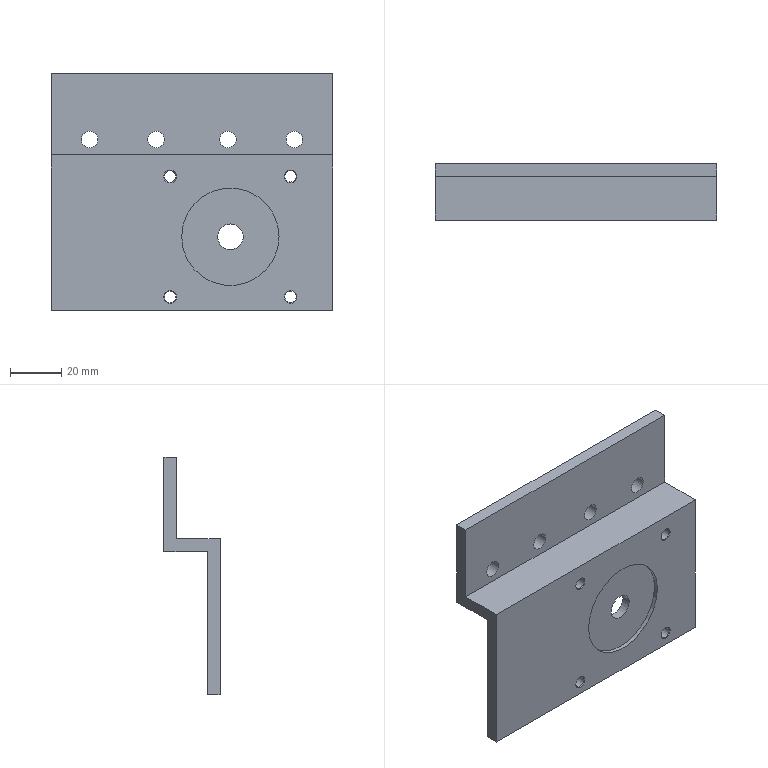Part | NX | features SIMPLE HOLE 10, DATUM_CSYS 5, SKETCH 4, SYMBOLIC_THREAD 4, HOLE PACKAGE 3, EXTRUDE 2 | 1 solid | 29 faces | box 110 x 22 x 93 mm | volume 57423 mm3 | plane 11 | cylinder 10 | cone 8 | commonest cylinder face diameters 4.5 x4 6.5 x4 10 x1 38.1 x1
STEP:
#1=CARTESIAN_POINT('',(38.55,0.,55.1));
#2=VERTEX_POINT('',#1);
#3=CARTESIAN_POINT('',(38.55,0.,52.6));
#4=DIRECTION('',(0.,1.,0.));
#5=DIRECTION('',(0.,0.,1.));
#6=AXIS2_PLACEMENT_3D('',#3,#4,#5);
#7=CIRCLE('',#6,2.5);
#8=EDGE_CURVE('',#2,#2,#7,.T.);
#9=ORIENTED_EDGE('',*,*,#8,.T.);
#10=EDGE_LOOP('',(#9));
#11=FACE_BOUND('',#10,.T.);
#12=CARTESIAN_POINT('',(38.55,0.,8.));
#13=VERTEX_POINT('',#12);
#14=CARTESIAN_POINT('',(38.55,0.,5.5));
#15=DIRECTION('',(0.,1.,0.));
#16=DIRECTION('',(0.,0.,1.));
#17=AXIS2_PLACEMENT_3D('',#14,#15,#16);
#18=CIRCLE('',#17,2.5);
#19=EDGE_CURVE('',#13,#13,#18,.T.);
#20=ORIENTED_EDGE('',*,*,#19,.T.);
#21=EDGE_LOOP('',(#20));
#22=FACE_BOUND('',#21,.T.);
#23=CARTESIAN_POINT('',(-8.55,0.,55.05));
#24=VERTEX_POINT('',#23);
#25=CARTESIAN_POINT('',(-8.55,0.,52.55));
#26=DIRECTION('',(0.,1.,0.));
#27=DIRECTION('',(0.,0.,1.));
#28=AXIS2_PLACEMENT_3D('',#25,#26,#27);
#29=CIRCLE('',#28,2.5);
#30=EDGE_CURVE('',#24,#24,#29,.T.);
#31=ORIENTED_EDGE('',*,*,#30,.T.);
#32=EDGE_LOOP('',(#31));
#33=FACE_BOUND('',#32,.T.);
#34=CARTESIAN_POINT('',(-8.55,0.,7.95));
#35=VERTEX_POINT('',#34);
#36=CARTESIAN_POINT('',(-8.55,0.,5.45));
#37=DIRECTION('',(0.,1.,0.));
#38=DIRECTION('',(0.,0.,1.));
#39=AXIS2_PLACEMENT_3D('',#36,#37,#38);
#40=CIRCLE('',#39,2.5);
#41=EDGE_CURVE('',#35,#35,#40,.T.);
#42=ORIENTED_EDGE('',*,*,#41,.T.);
#43=EDGE_LOOP('',(#42));
#44=FACE_BOUND('',#43,.T.);
#45=CARTESIAN_POINT('',(34.05,0.,29.));
#46=VERTEX_POINT('',#45);
#47=CARTESIAN_POINT('',(15.,0.,29.));
#48=DIRECTION('',(0.,-1.,0.));
#49=DIRECTION('',(1.,0.,0.));
#50=AXIS2_PLACEMENT_3D('',#47,#48,#49);
#51=CIRCLE('',#50,19.05);
#52=EDGE_CURVE('',#46,#46,#51,.T.);
#53=ORIENTED_EDGE('',*,*,#52,.F.);
#54=EDGE_LOOP('',(#53));
#55=FACE_BOUND('',#54,.T.);
#56=CARTESIAN_POINT('',(-55.,0.,61.));
#57=VERTEX_POINT('',#56);
#58=CARTESIAN_POINT('',(-55.,0.,0.));
#59=VERTEX_POINT('',#58);
#60=CARTESIAN_POINT('',(-55.,0.,61.));
#61=DIRECTION('',(0.,0.,-1.));
#62=VECTOR('',#61,1000.);
#63=LINE('',#60,#62);
#64=EDGE_CURVE('',#57,#59,#63,.T.);
#65=ORIENTED_EDGE('',*,*,#64,.T.);
#66=CARTESIAN_POINT('',(55.,0.,0.));
#67=VERTEX_POINT('',#66);
#68=CARTESIAN_POINT('',(55.,0.,0.));
#69=DIRECTION('',(-1.,0.,0.));
#70=VECTOR('',#69,1000.);
#71=LINE('',#68,#70);
#72=EDGE_CURVE('',#67,#59,#71,.T.);
#73=ORIENTED_EDGE('',*,*,#72,.F.);
#74=CARTESIAN_POINT('',(55.,0.,61.));
#75=VERTEX_POINT('',#74);
#76=CARTESIAN_POINT('',(55.,0.,61.));
#77=DIRECTION('',(0.,0.,-1.));
#78=VECTOR('',#77,1000.);
#79=LINE('',#76,#78);
#80=EDGE_CURVE('',#75,#67,#79,.T.);
#81=ORIENTED_EDGE('',*,*,#80,.F.);
#82=CARTESIAN_POINT('',(55.,0.,61.));
#83=DIRECTION('',(-1.,0.,0.));
#84=VECTOR('',#83,1000.);
#85=LINE('',#82,#84);
#86=EDGE_CURVE('',#75,#57,#85,.T.);
#87=ORIENTED_EDGE('',*,*,#86,.T.);
#88=EDGE_LOOP('',(#65,#73,#81,#87));
#89=FACE_BOUND('',#88,.T.);
#90=CARTESIAN_POINT('',(55.,0.,61.));
#91=DIRECTION('',(0.,1.,0.));
#92=DIRECTION('',(0.,0.,1.));
#93=AXIS2_PLACEMENT_3D('',#90,#91,#92);
#94=PLANE('',#93);
#95=ADVANCED_FACE('',(#11,#22,#33,#44,#55,#89),#94,.F.);
#96=CARTESIAN_POINT('',(-55.,5.,0.));
#97=VERTEX_POINT('',#96);
#98=CARTESIAN_POINT('',(-55.,0.,0.));
#99=DIRECTION('',(0.,1.,0.));
#100=VECTOR('',#99,1000.);
#101=LINE('',#98,#100);
#102=EDGE_CURVE('',#59,#97,#101,.T.);
#103=ORIENTED_EDGE('',*,*,#102,.T.);
#104=CARTESIAN_POINT('',(55.,5.,0.));
#105=VERTEX_POINT('',#104);
#106=CARTESIAN_POINT('',(55.,5.,0.));
#107=DIRECTION('',(-1.,0.,0.));
#108=VECTOR('',#107,1000.);
#109=LINE('',#106,#108);
#110=EDGE_CURVE('',#105,#97,#109,.T.);
#111=ORIENTED_EDGE('',*,*,#110,.F.);
#112=CARTESIAN_POINT('',(55.,0.,0.));
#113=DIRECTION('',(0.,1.,0.));
#114=VECTOR('',#113,1000.);
#115=LINE('',#112,#114);
#116=EDGE_CURVE('',#67,#105,#115,.T.);
#117=ORIENTED_EDGE('',*,*,#116,.F.);
#118=ORIENTED_EDGE('',*,*,#72,.T.);
#119=EDGE_LOOP('',(#103,#111,#117,#118));
#120=FACE_BOUND('',#119,.T.);
#121=CARTESIAN_POINT('',(55.,0.,0.));
#122=DIRECTION('',(0.,0.,1.));
#123=DIRECTION('',(0.,-1.,0.));
#124=AXIS2_PLACEMENT_3D('',#121,#122,#123);
#125=PLANE('',#124);
#126=ADVANCED_FACE('',(#120),#125,.F.);
#127=CARTESIAN_POINT('',(38.55,5.,50.1));
#128=VERTEX_POINT('',#127);
#129=CARTESIAN_POINT('',(38.55,5.,52.6));
#130=DIRECTION('',(0.,-1.,0.));
#131=DIRECTION('',(0.,0.,-1.));
#132=AXIS2_PLACEMENT_3D('',#129,#130,#131);
#133=CIRCLE('',#132,2.5);
#134=EDGE_CURVE('',#128,#128,#133,.T.);
#135=ORIENTED_EDGE('',*,*,#134,.T.);
#136=EDGE_LOOP('',(#135));
#137=FACE_BOUND('',#136,.T.);
#138=CARTESIAN_POINT('',(38.55,5.,3.));
#139=VERTEX_POINT('',#138);
#140=CARTESIAN_POINT('',(38.55,5.,5.5));
#141=DIRECTION('',(0.,-1.,0.));
#142=DIRECTION('',(0.,0.,-1.));
#143=AXIS2_PLACEMENT_3D('',#140,#141,#142);
#144=CIRCLE('',#143,2.5);
#145=EDGE_CURVE('',#139,#139,#144,.T.);
#146=ORIENTED_EDGE('',*,*,#145,.T.);
#147=EDGE_LOOP('',(#146));
#148=FACE_BOUND('',#147,.T.);
#149=CARTESIAN_POINT('',(-8.55,5.,50.05));
#150=VERTEX_POINT('',#149);
#151=CARTESIAN_POINT('',(-8.55,5.,52.55));
#152=DIRECTION('',(0.,-1.,0.));
#153=DIRECTION('',(0.,0.,-1.));
#154=AXIS2_PLACEMENT_3D('',#151,#152,#153);
#155=CIRCLE('',#154,2.5);
#156=EDGE_CURVE('',#150,#150,#155,.T.);
#157=ORIENTED_EDGE('',*,*,#156,.T.);
#158=EDGE_LOOP('',(#157));
#159=FACE_BOUND('',#158,.T.);
#160=CARTESIAN_POINT('',(-8.55,5.,2.95));
#161=VERTEX_POINT('',#160);
#162=CARTESIAN_POINT('',(-8.55,5.,5.45));
#163=DIRECTION('',(0.,-1.,0.));
#164=DIRECTION('',(0.,0.,-1.));
#165=AXIS2_PLACEMENT_3D('',#162,#163,#164);
#166=CIRCLE('',#165,2.5);
#167=EDGE_CURVE('',#161,#161,#166,.T.);
#168=ORIENTED_EDGE('',*,*,#167,.T.);
#169=EDGE_LOOP('',(#168));
#170=FACE_BOUND('',#169,.T.);
#171=CARTESIAN_POINT('',(15.,5.,24.));
#172=VERTEX_POINT('',#171);
#173=CARTESIAN_POINT('',(15.,5.,29.));
#174=DIRECTION('',(0.,-1.,0.));
#175=DIRECTION('',(0.,0.,-1.));
#176=AXIS2_PLACEMENT_3D('',#173,#174,#175);
#177=CIRCLE('',#176,5.);
#178=EDGE_CURVE('',#172,#172,#177,.T.);
#179=ORIENTED_EDGE('',*,*,#178,.T.);
#180=EDGE_LOOP('',(#179));
#181=FACE_BOUND('',#180,.T.);
#182=CARTESIAN_POINT('',(-55.,5.,56.));
#183=VERTEX_POINT('',#182);
#184=CARTESIAN_POINT('',(-55.,5.,0.));
#185=DIRECTION('',(0.,0.,1.));
#186=VECTOR('',#185,1000.);
#187=LINE('',#184,#186);
#188=EDGE_CURVE('',#97,#183,#187,.T.);
#189=ORIENTED_EDGE('',*,*,#188,.T.);
#190=CARTESIAN_POINT('',(55.,5.,56.));
#191=VERTEX_POINT('',#190);
#192=CARTESIAN_POINT('',(55.,5.,56.));
#193=DIRECTION('',(-1.,0.,0.));
#194=VECTOR('',#193,1000.);
#195=LINE('',#192,#194);
#196=EDGE_CURVE('',#191,#183,#195,.T.);
#197=ORIENTED_EDGE('',*,*,#196,.F.);
#198=CARTESIAN_POINT('',(55.,5.,0.));
#199=DIRECTION('',(0.,0.,1.));
#200=VECTOR('',#199,1000.);
#201=LINE('',#198,#200);
#202=EDGE_CURVE('',#105,#191,#201,.T.);
#203=ORIENTED_EDGE('',*,*,#202,.F.);
#204=ORIENTED_EDGE('',*,*,#110,.T.);
#205=EDGE_LOOP('',(#189,#197,#203,#204));
#206=FACE_BOUND('',#205,.T.);
#207=CARTESIAN_POINT('',(55.,5.,0.));
#208=DIRECTION('',(0.,-1.,0.));
#209=DIRECTION('',(0.,0.,-1.));
#210=AXIS2_PLACEMENT_3D('',#207,#208,#209);
#211=PLANE('',#210);
#212=ADVANCED_FACE('',(#137,#148,#159,#170,#181,#206),#211,.F.);
#213=CARTESIAN_POINT('',(-55.,22.,56.));
#214=VERTEX_POINT('',#213);
#215=CARTESIAN_POINT('',(-55.,5.,56.));
#216=DIRECTION('',(0.,1.,0.));
#217=VECTOR('',#216,1000.);
#218=LINE('',#215,#217);
#219=EDGE_CURVE('',#183,#214,#218,.T.);
#220=ORIENTED_EDGE('',*,*,#219,.T.);
#221=CARTESIAN_POINT('',(55.,22.,56.));
#222=VERTEX_POINT('',#221);
#223=CARTESIAN_POINT('',(55.,22.,56.));
#224=DIRECTION('',(-1.,0.,0.));
#225=VECTOR('',#224,1000.);
#226=LINE('',#223,#225);
#227=EDGE_CURVE('',#222,#214,#226,.T.);
#228=ORIENTED_EDGE('',*,*,#227,.F.);
#229=CARTESIAN_POINT('',(55.,5.,56.));
#230=DIRECTION('',(0.,1.,0.));
#231=VECTOR('',#230,1000.);
#232=LINE('',#229,#231);
#233=EDGE_CURVE('',#191,#222,#232,.T.);
#234=ORIENTED_EDGE('',*,*,#233,.F.);
#235=ORIENTED_EDGE('',*,*,#196,.T.);
#236=EDGE_LOOP('',(#220,#228,#234,#235));
#237=FACE_BOUND('',#236,.T.);
#238=CARTESIAN_POINT('',(55.,5.,56.));
#239=DIRECTION('',(0.,0.,1.));
#240=DIRECTION('',(1.,0.,0.));
#241=AXIS2_PLACEMENT_3D('',#238,#239,#240);
#242=PLANE('',#241);
#243=ADVANCED_FACE('',(#237),#242,.F.);
#244=CARTESIAN_POINT('',(40.,22.,63.75));
#245=VERTEX_POINT('',#244);
#246=CARTESIAN_POINT('',(40.,22.,67.));
#247=DIRECTION('',(0.,-1.,0.));
#248=DIRECTION('',(0.,0.,-1.));
#249=AXIS2_PLACEMENT_3D('',#246,#247,#248);
#250=CIRCLE('',#249,3.25);
#251=EDGE_CURVE('',#245,#245,#250,.T.);
#252=ORIENTED_EDGE('',*,*,#251,.T.);
#253=EDGE_LOOP('',(#252));
#254=FACE_BOUND('',#253,.T.);
#255=CARTESIAN_POINT('',(14.,22.,63.75));
#256=VERTEX_POINT('',#255);
#257=CARTESIAN_POINT('',(14.,22.,67.));
#258=DIRECTION('',(0.,-1.,0.));
#259=DIRECTION('',(0.,0.,-1.));
#260=AXIS2_PLACEMENT_3D('',#257,#258,#259);
#261=CIRCLE('',#260,3.25);
#262=EDGE_CURVE('',#256,#256,#261,.T.);
#263=ORIENTED_EDGE('',*,*,#262,.T.);
#264=EDGE_LOOP('',(#263));
#265=FACE_BOUND('',#264,.T.);
#266=CARTESIAN_POINT('',(-14.,22.,63.75));
#267=VERTEX_POINT('',#266);
#268=CARTESIAN_POINT('',(-14.,22.,67.));
#269=DIRECTION('',(0.,-1.,0.));
#270=DIRECTION('',(0.,0.,-1.));
#271=AXIS2_PLACEMENT_3D('',#268,#269,#270);
#272=CIRCLE('',#271,3.25);
#273=EDGE_CURVE('',#267,#267,#272,.T.);
#274=ORIENTED_EDGE('',*,*,#273,.T.);
#275=EDGE_LOOP('',(#274));
#276=FACE_BOUND('',#275,.T.);
#277=CARTESIAN_POINT('',(-40.,22.,63.75));
#278=VERTEX_POINT('',#277);
#279=CARTESIAN_POINT('',(-40.,22.,67.));
#280=DIRECTION('',(0.,-1.,0.));
#281=DIRECTION('',(0.,0.,-1.));
#282=AXIS2_PLACEMENT_3D('',#279,#280,#281);
#283=CIRCLE('',#282,3.25);
#284=EDGE_CURVE('',#278,#278,#283,.T.);
#285=ORIENTED_EDGE('',*,*,#284,.T.);
#286=EDGE_LOOP('',(#285));
#287=FACE_BOUND('',#286,.T.);
#288=CARTESIAN_POINT('',(-55.,22.,93.));
#289=VERTEX_POINT('',#288);
#290=CARTESIAN_POINT('',(-55.,22.,56.));
#291=DIRECTION('',(0.,0.,1.));
#292=VECTOR('',#291,1000.);
#293=LINE('',#290,#292);
#294=EDGE_CURVE('',#214,#289,#293,.T.);
#295=ORIENTED_EDGE('',*,*,#294,.T.);
#296=CARTESIAN_POINT('',(55.,22.,93.));
#297=VERTEX_POINT('',#296);
#298=CARTESIAN_POINT('',(55.,22.,93.));
#299=DIRECTION('',(-1.,0.,0.));
#300=VECTOR('',#299,1000.);
#301=LINE('',#298,#300);
#302=EDGE_CURVE('',#297,#289,#301,.T.);
#303=ORIENTED_EDGE('',*,*,#302,.F.);
#304=CARTESIAN_POINT('',(55.,22.,56.));
#305=DIRECTION('',(0.,0.,1.));
#306=VECTOR('',#305,1000.);
#307=LINE('',#304,#306);
#308=EDGE_CURVE('',#222,#297,#307,.T.);
#309=ORIENTED_EDGE('',*,*,#308,.F.);
#310=ORIENTED_EDGE('',*,*,#227,.T.);
#311=EDGE_LOOP('',(#295,#303,#309,#310));
#312=FACE_BOUND('',#311,.T.);
#313=CARTESIAN_POINT('',(55.,22.,56.));
#314=DIRECTION('',(0.,-1.,0.));
#315=DIRECTION('',(0.,0.,-1.));
#316=AXIS2_PLACEMENT_3D('',#313,#314,#315);
#317=PLANE('',#316);
#318=ADVANCED_FACE('',(#254,#265,#276,#287,#312),#317,.F.);
#319=CARTESIAN_POINT('',(-55.,17.,93.));
#320=VERTEX_POINT('',#319);
#321=CARTESIAN_POINT('',(-55.,22.,93.));
#322=DIRECTION('',(0.,-1.,0.));
#323=VECTOR('',#322,1000.);
#324=LINE('',#321,#323);
#325=EDGE_CURVE('',#289,#320,#324,.T.);
#326=ORIENTED_EDGE('',*,*,#325,.T.);
#327=CARTESIAN_POINT('',(55.,17.,93.));
#328=VERTEX_POINT('',#327);
#329=CARTESIAN_POINT('',(55.,17.,93.));
#330=DIRECTION('',(-1.,0.,0.));
#331=VECTOR('',#330,1000.);
#332=LINE('',#329,#331);
#333=EDGE_CURVE('',#328,#320,#332,.T.);
#334=ORIENTED_EDGE('',*,*,#333,.F.);
#335=CARTESIAN_POINT('',(55.,22.,93.));
#336=DIRECTION('',(0.,-1.,0.));
#337=VECTOR('',#336,1000.);
#338=LINE('',#335,#337);
#339=EDGE_CURVE('',#297,#328,#338,.T.);
#340=ORIENTED_EDGE('',*,*,#339,.F.);
#341=ORIENTED_EDGE('',*,*,#302,.T.);
#342=EDGE_LOOP('',(#326,#334,#340,#341));
#343=FACE_BOUND('',#342,.T.);
#344=CARTESIAN_POINT('',(55.,22.,93.));
#345=DIRECTION('',(0.,0.,-1.));
#346=DIRECTION('',(-1.,0.,0.));
#347=AXIS2_PLACEMENT_3D('',#344,#345,#346);
#348=PLANE('',#347);
#349=ADVANCED_FACE('',(#343),#348,.F.);
#350=CARTESIAN_POINT('',(40.,17.,70.25));
#351=VERTEX_POINT('',#350);
#352=CARTESIAN_POINT('',(40.,17.,67.));
#353=DIRECTION('',(0.,1.,0.));
#354=DIRECTION('',(0.,0.,1.));
#355=AXIS2_PLACEMENT_3D('',#352,#353,#354);
#356=CIRCLE('',#355,3.25);
#357=EDGE_CURVE('',#351,#351,#356,.T.);
#358=ORIENTED_EDGE('',*,*,#357,.T.);
#359=EDGE_LOOP('',(#358));
#360=FACE_BOUND('',#359,.T.);
#361=CARTESIAN_POINT('',(14.,17.,70.25));
#362=VERTEX_POINT('',#361);
#363=CARTESIAN_POINT('',(14.,17.,67.));
#364=DIRECTION('',(0.,1.,0.));
#365=DIRECTION('',(0.,0.,1.));
#366=AXIS2_PLACEMENT_3D('',#363,#364,#365);
#367=CIRCLE('',#366,3.25);
#368=EDGE_CURVE('',#362,#362,#367,.T.);
#369=ORIENTED_EDGE('',*,*,#368,.T.);
#370=EDGE_LOOP('',(#369));
#371=FACE_BOUND('',#370,.T.);
#372=CARTESIAN_POINT('',(-14.,17.,70.25));
#373=VERTEX_POINT('',#372);
#374=CARTESIAN_POINT('',(-14.,17.,67.));
#375=DIRECTION('',(0.,1.,0.));
#376=DIRECTION('',(0.,0.,1.));
#377=AXIS2_PLACEMENT_3D('',#374,#375,#376);
#378=CIRCLE('',#377,3.25);
#379=EDGE_CURVE('',#373,#373,#378,.T.);
#380=ORIENTED_EDGE('',*,*,#379,.T.);
#381=EDGE_LOOP('',(#380));
#382=FACE_BOUND('',#381,.T.);
#383=CARTESIAN_POINT('',(-40.,17.,70.25));
#384=VERTEX_POINT('',#383);
#385=CARTESIAN_POINT('',(-40.,17.,67.));
#386=DIRECTION('',(0.,1.,0.));
#387=DIRECTION('',(0.,0.,1.));
#388=AXIS2_PLACEMENT_3D('',#385,#386,#387);
#389=CIRCLE('',#388,3.25);
#390=EDGE_CURVE('',#384,#384,#389,.T.);
#391=ORIENTED_EDGE('',*,*,#390,.T.);
#392=EDGE_LOOP('',(#391));
#393=FACE_BOUND('',#392,.T.);
#394=CARTESIAN_POINT('',(-55.,17.,61.));
#395=VERTEX_POINT('',#394);
#396=CARTESIAN_POINT('',(-55.,17.,93.));
#397=DIRECTION('',(0.,0.,-1.));
#398=VECTOR('',#397,1000.);
#399=LINE('',#396,#398);
#400=EDGE_CURVE('',#320,#395,#399,.T.);
#401=ORIENTED_EDGE('',*,*,#400,.T.);
#402=CARTESIAN_POINT('',(55.,17.,61.));
#403=VERTEX_POINT('',#402);
#404=CARTESIAN_POINT('',(55.,17.,61.));
#405=DIRECTION('',(-1.,0.,0.));
#406=VECTOR('',#405,1000.);
#407=LINE('',#404,#406);
#408=EDGE_CURVE('',#403,#395,#407,.T.);
#409=ORIENTED_EDGE('',*,*,#408,.F.);
#410=CARTESIAN_POINT('',(55.,17.,93.));
#411=DIRECTION('',(0.,0.,-1.));
#412=VECTOR('',#411,1000.);
#413=LINE('',#410,#412);
#414=EDGE_CURVE('',#328,#403,#413,.T.);
#415=ORIENTED_EDGE('',*,*,#414,.F.);
#416=ORIENTED_EDGE('',*,*,#333,.T.);
#417=EDGE_LOOP('',(#401,#409,#415,#416));
#418=FACE_BOUND('',#417,.T.);
#419=CARTESIAN_POINT('',(55.,17.,93.));
#420=DIRECTION('',(0.,1.,0.));
#421=DIRECTION('',(0.,0.,1.));
#422=AXIS2_PLACEMENT_3D('',#419,#420,#421);
#423=PLANE('',#422);
#424=ADVANCED_FACE('',(#360,#371,#382,#393,#418),#423,.F.);
#425=CARTESIAN_POINT('',(-55.,17.,61.));
#426=DIRECTION('',(0.,-1.,0.));
#427=VECTOR('',#426,1000.);
#428=LINE('',#425,#427);
#429=EDGE_CURVE('',#395,#57,#428,.T.);
#430=ORIENTED_EDGE('',*,*,#429,.T.);
#431=ORIENTED_EDGE('',*,*,#86,.F.);
#432=CARTESIAN_POINT('',(55.,17.,61.));
#433=DIRECTION('',(0.,-1.,0.));
#434=VECTOR('',#433,1000.);
#435=LINE('',#432,#434);
#436=EDGE_CURVE('',#403,#75,#435,.T.);
#437=ORIENTED_EDGE('',*,*,#436,.F.);
#438=ORIENTED_EDGE('',*,*,#408,.T.);
#439=EDGE_LOOP('',(#430,#431,#437,#438));
#440=FACE_BOUND('',#439,.T.);
#441=CARTESIAN_POINT('',(55.,17.,61.));
#442=DIRECTION('',(0.,0.,-1.));
#443=DIRECTION('',(-1.,0.,0.));
#444=AXIS2_PLACEMENT_3D('',#441,#442,#443);
#445=PLANE('',#444);
#446=ADVANCED_FACE('',(#440),#445,.F.);
#447=ORIENTED_EDGE('',*,*,#80,.T.);
#448=ORIENTED_EDGE('',*,*,#116,.T.);
#449=ORIENTED_EDGE('',*,*,#202,.T.);
#450=ORIENTED_EDGE('',*,*,#233,.T.);
#451=ORIENTED_EDGE('',*,*,#308,.T.);
#452=ORIENTED_EDGE('',*,*,#339,.T.);
#453=ORIENTED_EDGE('',*,*,#414,.T.);
#454=ORIENTED_EDGE('',*,*,#436,.T.);
#455=EDGE_LOOP('',(#447,#448,#449,#450,#451,#452,#453,#454));
#456=FACE_BOUND('',#455,.T.);
#457=CARTESIAN_POINT('',(55.,0.,0.));
#458=DIRECTION('',(1.,0.,0.));
#459=DIRECTION('',(0.,0.,-1.));
#460=AXIS2_PLACEMENT_3D('',#457,#458,#459);
#461=PLANE('',#460);
#462=ADVANCED_FACE('',(#456),#461,.T.);
#463=ORIENTED_EDGE('',*,*,#64,.F.);
#464=ORIENTED_EDGE('',*,*,#429,.F.);
#465=ORIENTED_EDGE('',*,*,#400,.F.);
#466=ORIENTED_EDGE('',*,*,#325,.F.);
#467=ORIENTED_EDGE('',*,*,#294,.F.);
#468=ORIENTED_EDGE('',*,*,#219,.F.);
#469=ORIENTED_EDGE('',*,*,#188,.F.);
#470=ORIENTED_EDGE('',*,*,#102,.F.);
#471=EDGE_LOOP('',(#463,#464,#465,#466,#467,#468,#469,#470));
#472=FACE_BOUND('',#471,.T.);
#473=CARTESIAN_POINT('',(-55.,0.,0.));
#474=DIRECTION('',(1.,0.,0.));
#475=DIRECTION('',(0.,0.,-1.));
#476=AXIS2_PLACEMENT_3D('',#473,#474,#475);
#477=PLANE('',#476);
#478=ADVANCED_FACE('',(#472),#477,.F.);
#479=CARTESIAN_POINT('',(34.05,1.6,29.));
#480=VERTEX_POINT('',#479);
#481=CARTESIAN_POINT('',(15.,1.6,29.));
#482=DIRECTION('',(0.,-1.,0.));
#483=DIRECTION('',(1.,0.,0.));
#484=AXIS2_PLACEMENT_3D('',#481,#482,#483);
#485=CIRCLE('',#484,19.05);
#486=EDGE_CURVE('',#480,#480,#485,.F.);
#487=ORIENTED_EDGE('',*,*,#486,.T.);
#488=EDGE_LOOP('',(#487));
#489=FACE_BOUND('',#488,.T.);
#490=ORIENTED_EDGE('',*,*,#52,.T.);
#491=EDGE_LOOP('',(#490));
#492=FACE_BOUND('',#491,.T.);
#493=CARTESIAN_POINT('',(15.,1.6,29.));
#494=DIRECTION('',(0.,-1.,0.));
#495=DIRECTION('',(0.,0.,-1.));
#496=AXIS2_PLACEMENT_3D('',#493,#494,#495);
#497=CYLINDRICAL_SURFACE('',#496,19.05);
#498=ADVANCED_FACE('',(#489,#492),#497,.F.);
#499=CARTESIAN_POINT('',(15.,1.6,34.));
#500=VERTEX_POINT('',#499);
#501=CARTESIAN_POINT('',(15.,1.6,29.));
#502=DIRECTION('',(0.,1.,0.));
#503=DIRECTION('',(0.,0.,1.));
#504=AXIS2_PLACEMENT_3D('',#501,#502,#503);
#505=CIRCLE('',#504,5.);
#506=EDGE_CURVE('',#500,#500,#505,.T.);
#507=ORIENTED_EDGE('',*,*,#506,.T.);
#508=EDGE_LOOP('',(#507));
#509=FACE_BOUND('',#508,.T.);
#510=ORIENTED_EDGE('',*,*,#486,.F.);
#511=EDGE_LOOP('',(#510));
#512=FACE_BOUND('',#511,.T.);
#513=CARTESIAN_POINT('',(15.,1.6,29.));
#514=DIRECTION('',(0.,-1.,0.));
#515=DIRECTION('',(0.,0.,-1.));
#516=AXIS2_PLACEMENT_3D('',#513,#514,#515);
#517=PLANE('',#516);
#518=ADVANCED_FACE('',(#509,#512),#517,.T.);
#519=ORIENTED_EDGE('',*,*,#506,.F.);
#520=EDGE_LOOP('',(#519));
#521=FACE_BOUND('',#520,.T.);
#522=ORIENTED_EDGE('',*,*,#178,.F.);
#523=EDGE_LOOP('',(#522));
#524=FACE_BOUND('',#523,.T.);
#525=CARTESIAN_POINT('',(15.,1.6,29.));
#526=DIRECTION('',(0.,1.,0.));
#527=DIRECTION('',(0.,0.,1.));
#528=AXIS2_PLACEMENT_3D('',#525,#526,#527);
#529=CYLINDRICAL_SURFACE('',#528,5.);
#530=ADVANCED_FACE('',(#521,#524),#529,.F.);
#531=CARTESIAN_POINT('',(-8.55,4.75,3.2));
#532=VERTEX_POINT('',#531);
#533=CARTESIAN_POINT('',(-8.55,4.75,5.45));
#534=DIRECTION('',(0.,-1.,0.));
#535=DIRECTION('',(0.,0.,-1.));
#536=AXIS2_PLACEMENT_3D('',#533,#534,#535);
#537=CIRCLE('',#536,2.25);
#538=EDGE_CURVE('',#532,#532,#537,.F.);
#539=ORIENTED_EDGE('',*,*,#538,.T.);
#540=EDGE_LOOP('',(#539));
#541=FACE_BOUND('',#540,.T.);
#542=CARTESIAN_POINT('',(-8.55,0.25,7.7));
#543=VERTEX_POINT('',#542);
#544=CARTESIAN_POINT('',(-8.55,0.25,5.45));
#545=DIRECTION('',(0.,1.,0.));
#546=DIRECTION('',(0.,0.,1.));
#547=AXIS2_PLACEMENT_3D('',#544,#545,#546);
#548=CIRCLE('',#547,2.25);
#549=EDGE_CURVE('',#543,#543,#548,.F.);
#550=ORIENTED_EDGE('',*,*,#549,.T.);
#551=EDGE_LOOP('',(#550));
#552=FACE_BOUND('',#551,.T.);
#553=CARTESIAN_POINT('',(-8.55,0.,5.45));
#554=DIRECTION('',(0.,1.,0.));
#555=DIRECTION('',(0.,0.,1.));
#556=AXIS2_PLACEMENT_3D('',#553,#554,#555);
#557=CYLINDRICAL_SURFACE('',#556,2.25);
#558=ADVANCED_FACE('',(#541,#552),#557,.F.);
#559=ORIENTED_EDGE('',*,*,#549,.F.);
#560=EDGE_LOOP('',(#559));
#561=FACE_BOUND('',#560,.T.);
#562=ORIENTED_EDGE('',*,*,#41,.F.);
#563=EDGE_LOOP('',(#562));
#564=FACE_BOUND('',#563,.T.);
#565=CARTESIAN_POINT('',(-8.55,0.,5.45));
#566=DIRECTION('',(0.,-1.,0.));
#567=DIRECTION('',(0.,0.,-1.));
#568=AXIS2_PLACEMENT_3D('',#565,#566,#567);
#569=CONICAL_SURFACE('',#568,2.5,0.7854);
#570=ADVANCED_FACE('',(#561,#564),#569,.F.);
#571=ORIENTED_EDGE('',*,*,#538,.F.);
#572=EDGE_LOOP('',(#571));
#573=FACE_BOUND('',#572,.T.);
#574=ORIENTED_EDGE('',*,*,#167,.F.);
#575=EDGE_LOOP('',(#574));
#576=FACE_BOUND('',#575,.T.);
#577=CARTESIAN_POINT('',(-8.55,5.,5.45));
#578=DIRECTION('',(0.,1.,0.));
#579=DIRECTION('',(0.,0.,1.));
#580=AXIS2_PLACEMENT_3D('',#577,#578,#579);
#581=CONICAL_SURFACE('',#580,2.5,0.7854);
#582=ADVANCED_FACE('',(#573,#576),#581,.F.);
#583=CARTESIAN_POINT('',(-8.55,4.75,50.3));
#584=VERTEX_POINT('',#583);
#585=CARTESIAN_POINT('',(-8.55,4.75,52.55));
#586=DIRECTION('',(0.,-1.,0.));
#587=DIRECTION('',(0.,0.,-1.));
#588=AXIS2_PLACEMENT_3D('',#585,#586,#587);
#589=CIRCLE('',#588,2.25);
#590=EDGE_CURVE('',#584,#584,#589,.F.);
#591=ORIENTED_EDGE('',*,*,#590,.T.);
#592=EDGE_LOOP('',(#591));
#593=FACE_BOUND('',#592,.T.);
#594=CARTESIAN_POINT('',(-8.55,0.25,54.8));
#595=VERTEX_POINT('',#594);
#596=CARTESIAN_POINT('',(-8.55,0.25,52.55));
#597=DIRECTION('',(0.,1.,0.));
#598=DIRECTION('',(0.,0.,1.));
#599=AXIS2_PLACEMENT_3D('',#596,#597,#598);
#600=CIRCLE('',#599,2.25);
#601=EDGE_CURVE('',#595,#595,#600,.F.);
#602=ORIENTED_EDGE('',*,*,#601,.T.);
#603=EDGE_LOOP('',(#602));
#604=FACE_BOUND('',#603,.T.);
#605=CARTESIAN_POINT('',(-8.55,0.,52.55));
#606=DIRECTION('',(0.,1.,0.));
#607=DIRECTION('',(0.,0.,1.));
#608=AXIS2_PLACEMENT_3D('',#605,#606,#607);
#609=CYLINDRICAL_SURFACE('',#608,2.25);
#610=ADVANCED_FACE('',(#593,#604),#609,.F.);
#611=ORIENTED_EDGE('',*,*,#601,.F.);
#612=EDGE_LOOP('',(#611));
#613=FACE_BOUND('',#612,.T.);
#614=ORIENTED_EDGE('',*,*,#30,.F.);
#615=EDGE_LOOP('',(#614));
#616=FACE_BOUND('',#615,.T.);
#617=CARTESIAN_POINT('',(-8.55,0.,52.55));
#618=DIRECTION('',(0.,-1.,0.));
#619=DIRECTION('',(0.,0.,-1.));
#620=AXIS2_PLACEMENT_3D('',#617,#618,#619);
#621=CONICAL_SURFACE('',#620,2.5,0.7854);
#622=ADVANCED_FACE('',(#613,#616),#621,.F.);
#623=ORIENTED_EDGE('',*,*,#590,.F.);
#624=EDGE_LOOP('',(#623));
#625=FACE_BOUND('',#624,.T.);
#626=ORIENTED_EDGE('',*,*,#156,.F.);
#627=EDGE_LOOP('',(#626));
#628=FACE_BOUND('',#627,.T.);
#629=CARTESIAN_POINT('',(-8.55,5.,52.55));
#630=DIRECTION('',(0.,1.,0.));
#631=DIRECTION('',(0.,0.,1.));
#632=AXIS2_PLACEMENT_3D('',#629,#630,#631);
#633=CONICAL_SURFACE('',#632,2.5,0.7854);
#634=ADVANCED_FACE('',(#625,#628),#633,.F.);
#635=CARTESIAN_POINT('',(38.55,4.75,3.25));
#636=VERTEX_POINT('',#635);
#637=CARTESIAN_POINT('',(38.55,4.75,5.5));
#638=DIRECTION('',(0.,-1.,0.));
#639=DIRECTION('',(0.,0.,-1.));
#640=AXIS2_PLACEMENT_3D('',#637,#638,#639);
#641=CIRCLE('',#640,2.25);
#642=EDGE_CURVE('',#636,#636,#641,.F.);
#643=ORIENTED_EDGE('',*,*,#642,.T.);
#644=EDGE_LOOP('',(#643));
#645=FACE_BOUND('',#644,.T.);
#646=CARTESIAN_POINT('',(38.55,0.25,7.75));
#647=VERTEX_POINT('',#646);
#648=CARTESIAN_POINT('',(38.55,0.25,5.5));
#649=DIRECTION('',(0.,1.,0.));
#650=DIRECTION('',(0.,0.,1.));
#651=AXIS2_PLACEMENT_3D('',#648,#649,#650);
#652=CIRCLE('',#651,2.25);
#653=EDGE_CURVE('',#647,#647,#652,.F.);
#654=ORIENTED_EDGE('',*,*,#653,.T.);
#655=EDGE_LOOP('',(#654));
#656=FACE_BOUND('',#655,.T.);
#657=CARTESIAN_POINT('',(38.55,0.,5.5));
#658=DIRECTION('',(0.,1.,0.));
#659=DIRECTION('',(0.,0.,1.));
#660=AXIS2_PLACEMENT_3D('',#657,#658,#659);
#661=CYLINDRICAL_SURFACE('',#660,2.25);
#662=ADVANCED_FACE('',(#645,#656),#661,.F.);
#663=ORIENTED_EDGE('',*,*,#653,.F.);
#664=EDGE_LOOP('',(#663));
#665=FACE_BOUND('',#664,.T.);
#666=ORIENTED_EDGE('',*,*,#19,.F.);
#667=EDGE_LOOP('',(#666));
#668=FACE_BOUND('',#667,.T.);
#669=CARTESIAN_POINT('',(38.55,0.,5.5));
#670=DIRECTION('',(0.,-1.,0.));
#671=DIRECTION('',(0.,0.,-1.));
#672=AXIS2_PLACEMENT_3D('',#669,#670,#671);
#673=CONICAL_SURFACE('',#672,2.5,0.7854);
#674=ADVANCED_FACE('',(#665,#668),#673,.F.);
#675=ORIENTED_EDGE('',*,*,#642,.F.);
#676=EDGE_LOOP('',(#675));
#677=FACE_BOUND('',#676,.T.);
#678=ORIENTED_EDGE('',*,*,#145,.F.);
#679=EDGE_LOOP('',(#678));
#680=FACE_BOUND('',#679,.T.);
#681=CARTESIAN_POINT('',(38.55,5.,5.5));
#682=DIRECTION('',(0.,1.,0.));
#683=DIRECTION('',(0.,0.,1.));
#684=AXIS2_PLACEMENT_3D('',#681,#682,#683);
#685=CONICAL_SURFACE('',#684,2.5,0.7854);
#686=ADVANCED_FACE('',(#677,#680),#685,.F.);
#687=CARTESIAN_POINT('',(38.55,4.75,50.35));
#688=VERTEX_POINT('',#687);
#689=CARTESIAN_POINT('',(38.55,4.75,52.6));
#690=DIRECTION('',(0.,-1.,0.));
#691=DIRECTION('',(0.,0.,-1.));
#692=AXIS2_PLACEMENT_3D('',#689,#690,#691);
#693=CIRCLE('',#692,2.25);
#694=EDGE_CURVE('',#688,#688,#693,.F.);
#695=ORIENTED_EDGE('',*,*,#694,.T.);
#696=EDGE_LOOP('',(#695));
#697=FACE_BOUND('',#696,.T.);
#698=CARTESIAN_POINT('',(38.55,0.25,54.85));
#699=VERTEX_POINT('',#698);
#700=CARTESIAN_POINT('',(38.55,0.25,52.6));
#701=DIRECTION('',(0.,1.,0.));
#702=DIRECTION('',(0.,0.,1.));
#703=AXIS2_PLACEMENT_3D('',#700,#701,#702);
#704=CIRCLE('',#703,2.25);
#705=EDGE_CURVE('',#699,#699,#704,.F.);
#706=ORIENTED_EDGE('',*,*,#705,.T.);
#707=EDGE_LOOP('',(#706));
#708=FACE_BOUND('',#707,.T.);
#709=CARTESIAN_POINT('',(38.55,0.,52.6));
#710=DIRECTION('',(0.,1.,0.));
#711=DIRECTION('',(0.,0.,1.));
#712=AXIS2_PLACEMENT_3D('',#709,#710,#711);
#713=CYLINDRICAL_SURFACE('',#712,2.25);
#714=ADVANCED_FACE('',(#697,#708),#713,.F.);
#715=ORIENTED_EDGE('',*,*,#705,.F.);
#716=EDGE_LOOP('',(#715));
#717=FACE_BOUND('',#716,.T.);
#718=ORIENTED_EDGE('',*,*,#8,.F.);
#719=EDGE_LOOP('',(#718));
#720=FACE_BOUND('',#719,.T.);
#721=CARTESIAN_POINT('',(38.55,0.,52.6));
#722=DIRECTION('',(0.,-1.,0.));
#723=DIRECTION('',(0.,0.,-1.));
#724=AXIS2_PLACEMENT_3D('',#721,#722,#723);
#725=CONICAL_SURFACE('',#724,2.5,0.7854);
#726=ADVANCED_FACE('',(#717,#720),#725,.F.);
#727=ORIENTED_EDGE('',*,*,#694,.F.);
#728=EDGE_LOOP('',(#727));
#729=FACE_BOUND('',#728,.T.);
#730=ORIENTED_EDGE('',*,*,#134,.F.);
#731=EDGE_LOOP('',(#730));
#732=FACE_BOUND('',#731,.T.);
#733=CARTESIAN_POINT('',(38.55,5.,52.6));
#734=DIRECTION('',(0.,1.,0.));
#735=DIRECTION('',(0.,0.,1.));
#736=AXIS2_PLACEMENT_3D('',#733,#734,#735);
#737=CONICAL_SURFACE('',#736,2.5,0.7854);
#738=ADVANCED_FACE('',(#729,#732),#737,.F.);
#739=ORIENTED_EDGE('',*,*,#390,.F.);
#740=EDGE_LOOP('',(#739));
#741=FACE_BOUND('',#740,.T.);
#742=ORIENTED_EDGE('',*,*,#284,.F.);
#743=EDGE_LOOP('',(#742));
#744=FACE_BOUND('',#743,.T.);
#745=CARTESIAN_POINT('',(-40.,17.,67.));
#746=DIRECTION('',(0.,1.,0.));
#747=DIRECTION('',(0.,0.,1.));
#748=AXIS2_PLACEMENT_3D('',#745,#746,#747);
#749=CYLINDRICAL_SURFACE('',#748,3.25);
#750=ADVANCED_FACE('',(#741,#744),#749,.F.);
#751=ORIENTED_EDGE('',*,*,#379,.F.);
#752=EDGE_LOOP('',(#751));
#753=FACE_BOUND('',#752,.T.);
#754=ORIENTED_EDGE('',*,*,#273,.F.);
#755=EDGE_LOOP('',(#754));
#756=FACE_BOUND('',#755,.T.);
#757=CARTESIAN_POINT('',(-14.,17.,67.));
#758=DIRECTION('',(0.,1.,0.));
#759=DIRECTION('',(0.,0.,1.));
#760=AXIS2_PLACEMENT_3D('',#757,#758,#759);
#761=CYLINDRICAL_SURFACE('',#760,3.25);
#762=ADVANCED_FACE('',(#753,#756),#761,.F.);
#763=ORIENTED_EDGE('',*,*,#368,.F.);
#764=EDGE_LOOP('',(#763));
#765=FACE_BOUND('',#764,.T.);
#766=ORIENTED_EDGE('',*,*,#262,.F.);
#767=EDGE_LOOP('',(#766));
#768=FACE_BOUND('',#767,.T.);
#769=CARTESIAN_POINT('',(14.,17.,67.));
#770=DIRECTION('',(0.,1.,0.));
#771=DIRECTION('',(0.,0.,1.));
#772=AXIS2_PLACEMENT_3D('',#769,#770,#771);
#773=CYLINDRICAL_SURFACE('',#772,3.25);
#774=ADVANCED_FACE('',(#765,#768),#773,.F.);
#775=ORIENTED_EDGE('',*,*,#357,.F.);
#776=EDGE_LOOP('',(#775));
#777=FACE_BOUND('',#776,.T.);
#778=ORIENTED_EDGE('',*,*,#251,.F.);
#779=EDGE_LOOP('',(#778));
#780=FACE_BOUND('',#779,.T.);
#781=CARTESIAN_POINT('',(40.,17.,67.));
#782=DIRECTION('',(0.,1.,0.));
#783=DIRECTION('',(0.,0.,1.));
#784=AXIS2_PLACEMENT_3D('',#781,#782,#783);
#785=CYLINDRICAL_SURFACE('',#784,3.25);
#786=ADVANCED_FACE('',(#777,#780),#785,.F.);
#787=CLOSED_SHELL('',(#95,#126,#212,#243,#318,#349,#424,#446,#462,#478,#498,#518,#530,#558,#570,#582,#610,#622,#634,#662,#674,#686,#714,#726,#738,#750,#762,#774,#786));
#788=MANIFOLD_SOLID_BREP('',#787);
#789=(LENGTH_UNIT()NAMED_UNIT(*)SI_UNIT(.MILLI.,.METRE.));
#790=UNCERTAINTY_MEASURE_WITH_UNIT(LENGTH_MEASURE(0.00001),#789,'','');
#791=(NAMED_UNIT(*)PLANE_ANGLE_UNIT()SI_UNIT($,.RADIAN.));
#792=(NAMED_UNIT(*)SI_UNIT($,.STERADIAN.)SOLID_ANGLE_UNIT());
#793=(GEOMETRIC_REPRESENTATION_CONTEXT(3)GLOBAL_UNCERTAINTY_ASSIGNED_CONTEXT((#790))GLOBAL_UNIT_ASSIGNED_CONTEXT((#789,#791,#792))REPRESENTATION_CONTEXT('',''));
#794=ADVANCED_BREP_SHAPE_REPRESENTATION('',(#788),#793);